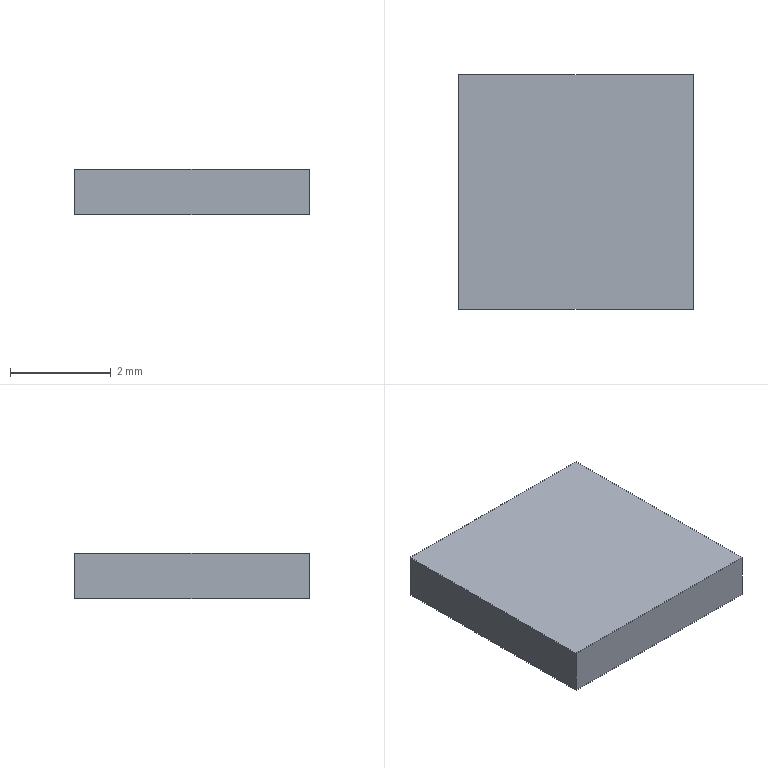Part | Creo | 1 solid | 6 faces | box 4.663 x 4.663 x 0.9 mm | volume 19.573 mm3 | plane 6
STEP:
#1=CARTESIAN_POINT('',(0.,0.,0.));
#2=DIRECTION('',(0.,0.,1.));
#3=DIRECTION('',(1.,0.,0.));
#4=AXIS2_PLACEMENT_3D('',#1,#2,#3);
#5=CARTESIAN_POINT('',(-2.364,-2.364,0.));
#6=VERTEX_POINT('',#5);
#7=CARTESIAN_POINT('',(2.3,-2.364,0.));
#8=VERTEX_POINT('',#7);
#9=CARTESIAN_POINT('',(-2.364,-2.364,0.));
#10=DIRECTION('',(1.,0.,0.));
#11=VECTOR('',#10,4.663);
#12=LINE('',#9,#11);
#13=EDGE_CURVE('',#6,#8,#12,.T.);
#14=ORIENTED_EDGE('',*,*,#13,.T.);
#15=CARTESIAN_POINT('',(2.3,2.3,0.));
#16=VERTEX_POINT('',#15);
#17=CARTESIAN_POINT('',(2.3,-2.364,0.));
#18=DIRECTION('',(0.,1.,0.));
#19=VECTOR('',#18,4.663);
#20=LINE('',#17,#19);
#21=EDGE_CURVE('',#8,#16,#20,.T.);
#22=ORIENTED_EDGE('',*,*,#21,.T.);
#23=CARTESIAN_POINT('',(-2.364,2.3,0.));
#24=VERTEX_POINT('',#23);
#25=CARTESIAN_POINT('',(2.3,2.3,0.));
#26=DIRECTION('',(-1.,0.,0.));
#27=VECTOR('',#26,4.663);
#28=LINE('',#25,#27);
#29=EDGE_CURVE('',#16,#24,#28,.T.);
#30=ORIENTED_EDGE('',*,*,#29,.T.);
#31=CARTESIAN_POINT('',(-2.364,2.3,0.));
#32=DIRECTION('',(0.,-1.,0.));
#33=VECTOR('',#32,4.663);
#34=LINE('',#31,#33);
#35=EDGE_CURVE('',#24,#6,#34,.T.);
#36=ORIENTED_EDGE('',*,*,#35,.T.);
#37=EDGE_LOOP('',(#14,#22,#30,#36));
#38=FACE_OUTER_BOUND('',#37,.F.);
#39=CARTESIAN_POINT('',(0.,0.,0.));
#40=DIRECTION('',(0.,0.,1.));
#41=DIRECTION('',(1.,0.,0.));
#42=AXIS2_PLACEMENT_3D('',#39,#40,#41);
#43=PLANE('',#42);
#44=ADVANCED_FACE('',(#38),#43,.F.);
#45=ORIENTED_EDGE('',*,*,#13,.F.);
#46=CARTESIAN_POINT('',(-2.364,-2.364,0.9));
#47=VERTEX_POINT('',#46);
#48=CARTESIAN_POINT('',(-2.364,-2.364,0.));
#49=DIRECTION('',(0.,0.,1.));
#50=VECTOR('',#49,0.9);
#51=LINE('',#48,#50);
#52=EDGE_CURVE('',#6,#47,#51,.T.);
#53=ORIENTED_EDGE('',*,*,#52,.T.);
#54=CARTESIAN_POINT('',(2.3,-2.364,0.9));
#55=VERTEX_POINT('',#54);
#56=CARTESIAN_POINT('',(-2.364,-2.364,0.9));
#57=DIRECTION('',(1.,0.,0.));
#58=VECTOR('',#57,4.663);
#59=LINE('',#56,#58);
#60=EDGE_CURVE('',#47,#55,#59,.T.);
#61=ORIENTED_EDGE('',*,*,#60,.T.);
#62=CARTESIAN_POINT('',(2.3,-2.364,0.));
#63=DIRECTION('',(0.,0.,1.));
#64=VECTOR('',#63,0.9);
#65=LINE('',#62,#64);
#66=EDGE_CURVE('',#8,#55,#65,.T.);
#67=ORIENTED_EDGE('',*,*,#66,.F.);
#68=EDGE_LOOP('',(#45,#53,#61,#67));
#69=FACE_OUTER_BOUND('',#68,.F.);
#70=CARTESIAN_POINT('',(-2.364,-2.364,0.));
#71=DIRECTION('',(0.,-1.,0.));
#72=DIRECTION('',(1.,0.,0.));
#73=AXIS2_PLACEMENT_3D('',#70,#71,#72);
#74=PLANE('',#73);
#75=ADVANCED_FACE('',(#69),#74,.T.);
#76=ORIENTED_EDGE('',*,*,#35,.F.);
#77=CARTESIAN_POINT('',(-2.364,2.3,0.9));
#78=VERTEX_POINT('',#77);
#79=CARTESIAN_POINT('',(-2.364,2.3,0.));
#80=DIRECTION('',(0.,0.,1.));
#81=VECTOR('',#80,0.9);
#82=LINE('',#79,#81);
#83=EDGE_CURVE('',#24,#78,#82,.T.);
#84=ORIENTED_EDGE('',*,*,#83,.T.);
#85=CARTESIAN_POINT('',(-2.364,2.3,0.9));
#86=DIRECTION('',(0.,-1.,0.));
#87=VECTOR('',#86,4.663);
#88=LINE('',#85,#87);
#89=EDGE_CURVE('',#78,#47,#88,.T.);
#90=ORIENTED_EDGE('',*,*,#89,.T.);
#91=ORIENTED_EDGE('',*,*,#52,.F.);
#92=EDGE_LOOP('',(#76,#84,#90,#91));
#93=FACE_OUTER_BOUND('',#92,.F.);
#94=CARTESIAN_POINT('',(-2.364,2.3,0.));
#95=DIRECTION('',(-1.,0.,0.));
#96=DIRECTION('',(0.,-1.,0.));
#97=AXIS2_PLACEMENT_3D('',#94,#95,#96);
#98=PLANE('',#97);
#99=ADVANCED_FACE('',(#93),#98,.T.);
#100=ORIENTED_EDGE('',*,*,#29,.F.);
#101=CARTESIAN_POINT('',(2.3,2.3,0.9));
#102=VERTEX_POINT('',#101);
#103=CARTESIAN_POINT('',(2.3,2.3,0.));
#104=DIRECTION('',(0.,0.,1.));
#105=VECTOR('',#104,0.9);
#106=LINE('',#103,#105);
#107=EDGE_CURVE('',#16,#102,#106,.T.);
#108=ORIENTED_EDGE('',*,*,#107,.T.);
#109=CARTESIAN_POINT('',(2.3,2.3,0.9));
#110=DIRECTION('',(-1.,0.,0.));
#111=VECTOR('',#110,4.663);
#112=LINE('',#109,#111);
#113=EDGE_CURVE('',#102,#78,#112,.T.);
#114=ORIENTED_EDGE('',*,*,#113,.T.);
#115=ORIENTED_EDGE('',*,*,#83,.F.);
#116=EDGE_LOOP('',(#100,#108,#114,#115));
#117=FACE_OUTER_BOUND('',#116,.F.);
#118=CARTESIAN_POINT('',(2.3,2.3,0.));
#119=DIRECTION('',(0.,1.,0.));
#120=DIRECTION('',(-1.,0.,0.));
#121=AXIS2_PLACEMENT_3D('',#118,#119,#120);
#122=PLANE('',#121);
#123=ADVANCED_FACE('',(#117),#122,.T.);
#124=ORIENTED_EDGE('',*,*,#21,.F.);
#125=ORIENTED_EDGE('',*,*,#66,.T.);
#126=CARTESIAN_POINT('',(2.3,-2.364,0.9));
#127=DIRECTION('',(0.,1.,0.));
#128=VECTOR('',#127,4.663);
#129=LINE('',#126,#128);
#130=EDGE_CURVE('',#55,#102,#129,.T.);
#131=ORIENTED_EDGE('',*,*,#130,.T.);
#132=ORIENTED_EDGE('',*,*,#107,.F.);
#133=EDGE_LOOP('',(#124,#125,#131,#132));
#134=FACE_OUTER_BOUND('',#133,.F.);
#135=CARTESIAN_POINT('',(2.3,-2.364,0.));
#136=DIRECTION('',(1.,0.,0.));
#137=DIRECTION('',(0.,1.,0.));
#138=AXIS2_PLACEMENT_3D('',#135,#136,#137);
#139=PLANE('',#138);
#140=ADVANCED_FACE('',(#134),#139,.T.);
#141=ORIENTED_EDGE('',*,*,#60,.F.);
#142=ORIENTED_EDGE('',*,*,#89,.F.);
#143=ORIENTED_EDGE('',*,*,#113,.F.);
#144=ORIENTED_EDGE('',*,*,#130,.F.);
#145=EDGE_LOOP('',(#141,#142,#143,#144));
#146=FACE_OUTER_BOUND('',#145,.F.);
#147=CARTESIAN_POINT('',(0.,0.,0.9));
#148=DIRECTION('',(0.,0.,1.));
#149=DIRECTION('',(1.,0.,0.));
#150=AXIS2_PLACEMENT_3D('',#147,#148,#149);
#151=PLANE('',#150);
#152=ADVANCED_FACE('',(#146),#151,.T.);
#153=CLOSED_SHELL('',(#44,#75,#99,#123,#140,#152));
#154=MANIFOLD_SOLID_BREP('',#153);
#155=(LENGTH_UNIT()NAMED_UNIT(*)SI_UNIT(.MILLI.,.METRE.));
#156=UNCERTAINTY_MEASURE_WITH_UNIT(LENGTH_MEASURE(0.0006656),#155,'','');
#157=(NAMED_UNIT(*)PLANE_ANGLE_UNIT()SI_UNIT($,.RADIAN.));
#158=PLANE_ANGLE_MEASURE_WITH_UNIT(PLANE_ANGLE_MEASURE(0.01745),#157);
#159=(CONVERSION_BASED_UNIT('DEGREE',#158)NAMED_UNIT(*)PLANE_ANGLE_UNIT());
#160=(NAMED_UNIT(*)SI_UNIT($,.STERADIAN.)SOLID_ANGLE_UNIT());
#161=(GEOMETRIC_REPRESENTATION_CONTEXT(3)GLOBAL_UNCERTAINTY_ASSIGNED_CONTEXT((#156))GLOBAL_UNIT_ASSIGNED_CONTEXT((#155,#159,#160))REPRESENTATION_CONTEXT('',''));
#162=ADVANCED_BREP_SHAPE_REPRESENTATION('',(#4,#154),#161);